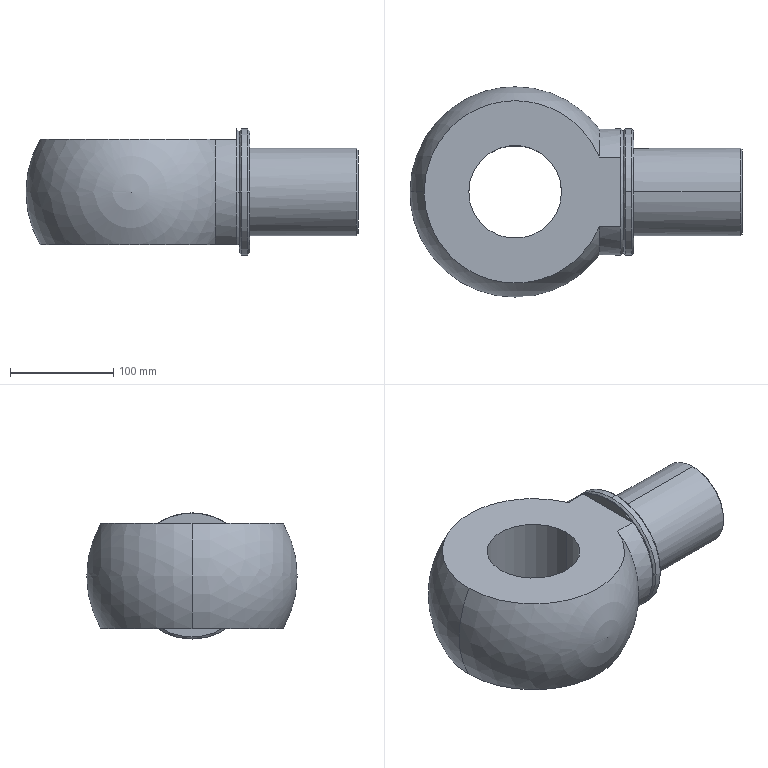Part | SolidWorks | features BaseBody 1 | 1 solid | 24 faces | box 322 x 204 x 122.4 mm | volume 3250841 mm3 | cone 9 | cylinder 7 | plane 6 | sphere 2 | commonest cylinder face diameters 122.4 x3 85 x2 90 x2
STEP:
#1=CARTESIAN_POINT('',(68.376,-42.5,0.));
#2=VERTEX_POINT('',#1);
#3=CARTESIAN_POINT('',(68.376,0.,42.5));
#4=VERTEX_POINT('',#3);
#5=CARTESIAN_POINT('',(68.376,0.,0.));
#6=DIRECTION('',(-1.,0.,0.));
#7=DIRECTION('',(0.,0.,-1.));
#8=AXIS2_PLACEMENT_3D('',#5,#6,#7);
#9=CIRCLE('',#8,42.5);
#10=EDGE_CURVE('',#2,#4,#9,.T.);
#11=ORIENTED_EDGE('',*,*,#10,.T.);
#12=CARTESIAN_POINT('',(-35.,0.,42.5));
#13=VERTEX_POINT('',#12);
#14=CARTESIAN_POINT('',(17.,0.,42.5));
#15=DIRECTION('',(-1.,0.,0.));
#16=VECTOR('',#15,1000.);
#17=LINE('',#14,#16);
#18=EDGE_CURVE('',#4,#13,#17,.T.);
#19=ORIENTED_EDGE('',*,*,#18,.T.);
#20=CARTESIAN_POINT('',(-35.,0.,-42.5));
#21=VERTEX_POINT('',#20);
#22=CARTESIAN_POINT('',(-35.,0.,0.));
#23=DIRECTION('',(-1.,0.,0.));
#24=DIRECTION('',(0.,0.,-1.));
#25=AXIS2_PLACEMENT_3D('',#22,#23,#24);
#26=CIRCLE('',#25,42.5);
#27=EDGE_CURVE('',#21,#13,#26,.T.);
#28=ORIENTED_EDGE('',*,*,#27,.F.);
#29=CARTESIAN_POINT('',(68.376,0.,-42.5));
#30=VERTEX_POINT('',#29);
#31=CARTESIAN_POINT('',(17.,0.,-42.5));
#32=DIRECTION('',(-1.,0.,0.));
#33=VECTOR('',#32,1000.);
#34=LINE('',#31,#33);
#35=EDGE_CURVE('',#30,#21,#34,.T.);
#36=ORIENTED_EDGE('',*,*,#35,.F.);
#37=CARTESIAN_POINT('',(68.376,0.,0.));
#38=DIRECTION('',(-1.,0.,0.));
#39=DIRECTION('',(0.,0.,-1.));
#40=AXIS2_PLACEMENT_3D('',#37,#38,#39);
#41=CIRCLE('',#40,42.5);
#42=EDGE_CURVE('',#30,#2,#41,.T.);
#43=ORIENTED_EDGE('',*,*,#42,.T.);
#44=EDGE_LOOP('',(#11,#19,#28,#36,#43));
#45=FACE_OUTER_BOUND('',#44,.T.);
#46=CARTESIAN_POINT('',(17.,0.,0.));
#47=DIRECTION('',(-1.,0.,0.));
#48=DIRECTION('',(0.,0.,-1.));
#49=AXIS2_PLACEMENT_3D('',#46,#47,#48);
#50=CYLINDRICAL_SURFACE('',#49,42.5);
#51=ADVANCED_FACE('',(#45),#50,.T.);
#52=CARTESIAN_POINT('',(70.,-40.876,0.));
#53=VERTEX_POINT('',#52);
#54=CARTESIAN_POINT('',(70.,40.876,0.));
#55=VERTEX_POINT('',#54);
#56=CARTESIAN_POINT('',(70.,0.,0.));
#57=DIRECTION('',(1.,0.,0.));
#58=DIRECTION('',(0.,1.,0.));
#59=AXIS2_PLACEMENT_3D('',#56,#57,#58);
#60=CIRCLE('',#59,40.876);
#61=EDGE_CURVE('',#53,#55,#60,.T.);
#62=ORIENTED_EDGE('',*,*,#61,.F.);
#63=CARTESIAN_POINT('',(69.188,-41.688,0.));
#64=DIRECTION('',(-0.7071,-0.7071,0.));
#65=VECTOR('',#64,1000.);
#66=LINE('',#63,#65);
#67=EDGE_CURVE('',#53,#2,#66,.T.);
#68=ORIENTED_EDGE('',*,*,#67,.T.);
#69=ORIENTED_EDGE('',*,*,#42,.F.);
#70=CARTESIAN_POINT('',(68.376,42.5,0.));
#71=VERTEX_POINT('',#70);
#72=CARTESIAN_POINT('',(68.376,0.,0.));
#73=DIRECTION('',(-1.,0.,0.));
#74=DIRECTION('',(0.,0.,-1.));
#75=AXIS2_PLACEMENT_3D('',#72,#73,#74);
#76=CIRCLE('',#75,42.5);
#77=EDGE_CURVE('',#71,#30,#76,.T.);
#78=ORIENTED_EDGE('',*,*,#77,.F.);
#79=CARTESIAN_POINT('',(69.188,41.688,0.));
#80=DIRECTION('',(-0.7071,0.7071,0.));
#81=VECTOR('',#80,1000.);
#82=LINE('',#79,#81);
#83=EDGE_CURVE('',#55,#71,#82,.T.);
#84=ORIENTED_EDGE('',*,*,#83,.F.);
#85=EDGE_LOOP('',(#62,#68,#69,#78,#84));
#86=FACE_OUTER_BOUND('',#85,.T.);
#87=CARTESIAN_POINT('',(69.188,0.,0.));
#88=DIRECTION('',(-1.,0.,0.));
#89=DIRECTION('',(0.,1.,0.));
#90=AXIS2_PLACEMENT_3D('',#87,#88,#89);
#91=CONICAL_SURFACE('',#90,41.688,0.7854);
#92=ADVANCED_FACE('',(#86),#91,.T.);
#93=CARTESIAN_POINT('',(-35.,-59.2,0.));
#94=VERTEX_POINT('',#93);
#95=CARTESIAN_POINT('',(-35.,59.2,0.));
#96=VERTEX_POINT('',#95);
#97=CARTESIAN_POINT('',(-35.,0.,0.));
#98=DIRECTION('',(1.,0.,0.));
#99=DIRECTION('',(0.,1.,0.));
#100=AXIS2_PLACEMENT_3D('',#97,#98,#99);
#101=CIRCLE('',#100,59.2);
#102=EDGE_CURVE('',#94,#96,#101,.T.);
#103=ORIENTED_EDGE('',*,*,#102,.F.);
#104=CARTESIAN_POINT('',(-37.,-61.2,0.));
#105=VERTEX_POINT('',#104);
#106=CARTESIAN_POINT('',(-36.,-60.2,0.));
#107=DIRECTION('',(-0.7071,-0.7071,0.));
#108=VECTOR('',#107,1000.);
#109=LINE('',#106,#108);
#110=EDGE_CURVE('',#94,#105,#109,.T.);
#111=ORIENTED_EDGE('',*,*,#110,.T.);
#112=CARTESIAN_POINT('',(-37.,0.,-61.2));
#113=VERTEX_POINT('',#112);
#114=CARTESIAN_POINT('',(-37.,0.,0.));
#115=DIRECTION('',(-1.,0.,0.));
#116=DIRECTION('',(0.,0.,-1.));
#117=AXIS2_PLACEMENT_3D('',#114,#115,#116);
#118=CIRCLE('',#117,61.2);
#119=EDGE_CURVE('',#113,#105,#118,.T.);
#120=ORIENTED_EDGE('',*,*,#119,.F.);
#121=CARTESIAN_POINT('',(-37.,61.2,0.));
#122=VERTEX_POINT('',#121);
#123=CARTESIAN_POINT('',(-37.,0.,0.));
#124=DIRECTION('',(-1.,0.,0.));
#125=DIRECTION('',(0.,0.,-1.));
#126=AXIS2_PLACEMENT_3D('',#123,#124,#125);
#127=CIRCLE('',#126,61.2);
#128=EDGE_CURVE('',#122,#113,#127,.T.);
#129=ORIENTED_EDGE('',*,*,#128,.F.);
#130=CARTESIAN_POINT('',(-36.,60.2,0.));
#131=DIRECTION('',(-0.7071,0.7071,0.));
#132=VECTOR('',#131,1000.);
#133=LINE('',#130,#132);
#134=EDGE_CURVE('',#96,#122,#133,.T.);
#135=ORIENTED_EDGE('',*,*,#134,.F.);
#136=EDGE_LOOP('',(#103,#111,#120,#129,#135));
#137=FACE_OUTER_BOUND('',#136,.T.);
#138=CARTESIAN_POINT('',(-36.,0.,0.));
#139=DIRECTION('',(-1.,0.,0.));
#140=DIRECTION('',(0.,1.,0.));
#141=AXIS2_PLACEMENT_3D('',#138,#139,#140);
#142=CONICAL_SURFACE('',#141,60.2,0.7854);
#143=ADVANCED_FACE('',(#137),#142,.T.);
#144=CARTESIAN_POINT('',(-45.,-59.2,0.));
#145=VERTEX_POINT('',#144);
#146=CARTESIAN_POINT('',(-45.,59.2,0.));
#147=VERTEX_POINT('',#146);
#148=CARTESIAN_POINT('',(-45.,0.,0.));
#149=DIRECTION('',(-1.,0.,0.));
#150=DIRECTION('',(0.,1.,0.));
#151=AXIS2_PLACEMENT_3D('',#148,#149,#150);
#152=CIRCLE('',#151,59.2);
#153=EDGE_CURVE('',#145,#147,#152,.T.);
#154=ORIENTED_EDGE('',*,*,#153,.F.);
#155=CARTESIAN_POINT('',(-43.,-61.2,0.));
#156=VERTEX_POINT('',#155);
#157=CARTESIAN_POINT('',(-44.,-60.2,0.));
#158=DIRECTION('',(0.7071,-0.7071,0.));
#159=VECTOR('',#158,1000.);
#160=LINE('',#157,#159);
#161=EDGE_CURVE('',#145,#156,#160,.T.);
#162=ORIENTED_EDGE('',*,*,#161,.T.);
#163=CARTESIAN_POINT('',(-43.,0.,61.2));
#164=VERTEX_POINT('',#163);
#165=CARTESIAN_POINT('',(-43.,0.,0.));
#166=DIRECTION('',(1.,0.,0.));
#167=DIRECTION('',(0.,0.,-1.));
#168=AXIS2_PLACEMENT_3D('',#165,#166,#167);
#169=CIRCLE('',#168,61.2);
#170=EDGE_CURVE('',#164,#156,#169,.T.);
#171=ORIENTED_EDGE('',*,*,#170,.F.);
#172=CARTESIAN_POINT('',(-43.,61.2,0.));
#173=VERTEX_POINT('',#172);
#174=CARTESIAN_POINT('',(-43.,0.,0.));
#175=DIRECTION('',(1.,0.,0.));
#176=DIRECTION('',(0.,0.,-1.));
#177=AXIS2_PLACEMENT_3D('',#174,#175,#176);
#178=CIRCLE('',#177,61.2);
#179=EDGE_CURVE('',#173,#164,#178,.T.);
#180=ORIENTED_EDGE('',*,*,#179,.F.);
#181=CARTESIAN_POINT('',(-44.,60.2,0.));
#182=DIRECTION('',(0.7071,0.7071,0.));
#183=VECTOR('',#182,1000.);
#184=LINE('',#181,#183);
#185=EDGE_CURVE('',#147,#173,#184,.T.);
#186=ORIENTED_EDGE('',*,*,#185,.F.);
#187=EDGE_LOOP('',(#154,#162,#171,#180,#186));
#188=FACE_OUTER_BOUND('',#187,.T.);
#189=CARTESIAN_POINT('',(-44.,0.,0.));
#190=DIRECTION('',(1.,0.,0.));
#191=DIRECTION('',(0.,1.,0.));
#192=AXIS2_PLACEMENT_3D('',#189,#190,#191);
#193=CONICAL_SURFACE('',#192,60.2,0.7854);
#194=ADVANCED_FACE('',(#188),#193,.T.);
#195=ORIENTED_EDGE('',*,*,#119,.T.);
#196=CARTESIAN_POINT('',(-37.,0.,61.2));
#197=VERTEX_POINT('',#196);
#198=CARTESIAN_POINT('',(-37.,0.,0.));
#199=DIRECTION('',(-1.,0.,0.));
#200=DIRECTION('',(0.,0.,-1.));
#201=AXIS2_PLACEMENT_3D('',#198,#199,#200);
#202=CIRCLE('',#201,61.2);
#203=EDGE_CURVE('',#105,#197,#202,.T.);
#204=ORIENTED_EDGE('',*,*,#203,.T.);
#205=CARTESIAN_POINT('',(-40.,0.,61.2));
#206=DIRECTION('',(-1.,0.,0.));
#207=VECTOR('',#206,1000.);
#208=LINE('',#205,#207);
#209=EDGE_CURVE('',#197,#164,#208,.T.);
#210=ORIENTED_EDGE('',*,*,#209,.T.);
#211=ORIENTED_EDGE('',*,*,#170,.T.);
#212=CARTESIAN_POINT('',(-43.,0.,-61.2));
#213=VERTEX_POINT('',#212);
#214=CARTESIAN_POINT('',(-43.,0.,0.));
#215=DIRECTION('',(1.,0.,0.));
#216=DIRECTION('',(0.,0.,-1.));
#217=AXIS2_PLACEMENT_3D('',#214,#215,#216);
#218=CIRCLE('',#217,61.2);
#219=EDGE_CURVE('',#156,#213,#218,.T.);
#220=ORIENTED_EDGE('',*,*,#219,.T.);
#221=CARTESIAN_POINT('',(-40.,0.,-61.2));
#222=DIRECTION('',(-1.,0.,0.));
#223=VECTOR('',#222,1000.);
#224=LINE('',#221,#223);
#225=EDGE_CURVE('',#113,#213,#224,.T.);
#226=ORIENTED_EDGE('',*,*,#225,.F.);
#227=EDGE_LOOP('',(#195,#204,#210,#211,#220,#226));
#228=FACE_OUTER_BOUND('',#227,.T.);
#229=CARTESIAN_POINT('',(-40.,0.,0.));
#230=DIRECTION('',(-1.,0.,0.));
#231=DIRECTION('',(0.,0.,-1.));
#232=AXIS2_PLACEMENT_3D('',#229,#230,#231);
#233=CYLINDRICAL_SURFACE('',#232,61.2);
#234=ADVANCED_FACE('',(#228),#233,.T.);
#235=CARTESIAN_POINT('',(-105.,0.,-51.));
#236=VERTEX_POINT('',#235);
#237=CARTESIAN_POINT('',(-195.,0.,-51.));
#238=VERTEX_POINT('',#237);
#239=CARTESIAN_POINT('',(-150.,0.,-51.));
#240=DIRECTION('',(0.,0.,1.));
#241=DIRECTION('',(-1.,0.,0.));
#242=AXIS2_PLACEMENT_3D('',#239,#240,#241);
#243=CIRCLE('',#242,45.);
#244=EDGE_CURVE('',#236,#238,#243,.T.);
#245=ORIENTED_EDGE('',*,*,#244,.F.);
#246=CARTESIAN_POINT('',(-105.,0.,51.));
#247=VERTEX_POINT('',#246);
#248=CARTESIAN_POINT('',(-105.,0.,0.));
#249=DIRECTION('',(0.,0.,1.));
#250=VECTOR('',#249,1000.);
#251=LINE('',#248,#250);
#252=EDGE_CURVE('',#236,#247,#251,.T.);
#253=ORIENTED_EDGE('',*,*,#252,.T.);
#254=CARTESIAN_POINT('',(-195.,0.,51.));
#255=VERTEX_POINT('',#254);
#256=CARTESIAN_POINT('',(-150.,0.,51.));
#257=DIRECTION('',(0.,0.,-1.));
#258=DIRECTION('',(-1.,0.,0.));
#259=AXIS2_PLACEMENT_3D('',#256,#257,#258);
#260=CIRCLE('',#259,45.);
#261=EDGE_CURVE('',#255,#247,#260,.T.);
#262=ORIENTED_EDGE('',*,*,#261,.F.);
#263=CARTESIAN_POINT('',(-195.,0.,0.));
#264=DIRECTION('',(0.,0.,1.));
#265=VECTOR('',#264,1000.);
#266=LINE('',#263,#265);
#267=EDGE_CURVE('',#238,#255,#266,.T.);
#268=ORIENTED_EDGE('',*,*,#267,.F.);
#269=EDGE_LOOP('',(#245,#253,#262,#268));
#270=FACE_OUTER_BOUND('',#269,.T.);
#271=CARTESIAN_POINT('',(-150.,0.,0.));
#272=DIRECTION('',(0.,0.,1.));
#273=DIRECTION('',(-1.,0.,0.));
#274=AXIS2_PLACEMENT_3D('',#271,#272,#273);
#275=CYLINDRICAL_SURFACE('',#274,45.);
#276=ADVANCED_FACE('',(#270),#275,.F.);
#277=CARTESIAN_POINT('',(-45.,-58.752,0.));
#278=VERTEX_POINT('',#277);
#279=CARTESIAN_POINT('',(-45.,-29.168,-51.));
#280=VERTEX_POINT('',#279);
#281=CARTESIAN_POINT('',(-45.,0.,0.));
#282=DIRECTION('',(1.,0.,0.));
#283=DIRECTION('',(0.,1.,0.));
#284=AXIS2_PLACEMENT_3D('',#281,#282,#283);
#285=CIRCLE('',#284,58.752);
#286=EDGE_CURVE('',#278,#280,#285,.T.);
#287=ORIENTED_EDGE('',*,*,#286,.F.);
#288=CARTESIAN_POINT('',(-47.448,-61.2,0.));
#289=VERTEX_POINT('',#288);
#290=CARTESIAN_POINT('',(-46.224,-59.976,0.));
#291=DIRECTION('',(-0.7071,-0.7071,0.));
#292=VECTOR('',#291,1000.);
#293=LINE('',#290,#292);
#294=EDGE_CURVE('',#278,#289,#293,.T.);
#295=ORIENTED_EDGE('',*,*,#294,.T.);
#296=CARTESIAN_POINT('',(-47.448,-33.83,-51.));
#297=VERTEX_POINT('',#296);
#298=CARTESIAN_POINT('',(-47.448,0.,0.));
#299=DIRECTION('',(-1.,0.,0.));
#300=DIRECTION('',(0.,0.,-1.));
#301=AXIS2_PLACEMENT_3D('',#298,#299,#300);
#302=CIRCLE('',#301,61.2);
#303=EDGE_CURVE('',#297,#289,#302,.T.);
#304=ORIENTED_EDGE('',*,*,#303,.F.);
#305=CARTESIAN_POINT('',(-47.448,-33.83,-51.));
#306=CARTESIAN_POINT('',(-46.133,-31.451,-51.));
#307=CARTESIAN_POINT('',(-45.,-29.168,-51.));
#308=(BOUNDED_CURVE()B_SPLINE_CURVE(2,(#305,#306,#307),.UNSPECIFIED.,.F.,.F.)B_SPLINE_CURVE_WITH_KNOTS((3,3),(0.,5.265),.UNSPECIFIED.)CURVE()GEOMETRIC_REPRESENTATION_ITEM()RATIONAL_B_SPLINE_CURVE((1.,1.001,1.))REPRESENTATION_ITEM(''));
#309=EDGE_CURVE('',#297,#280,#308,.T.);
#310=ORIENTED_EDGE('',*,*,#309,.T.);
#311=EDGE_LOOP('',(#287,#295,#304,#310));
#312=FACE_OUTER_BOUND('',#311,.T.);
#313=CARTESIAN_POINT('',(-46.224,0.,0.));
#314=DIRECTION('',(-1.,0.,0.));
#315=DIRECTION('',(0.,1.,0.));
#316=AXIS2_PLACEMENT_3D('',#313,#314,#315);
#317=CONICAL_SURFACE('',#316,59.976,0.7854);
#318=ADVANCED_FACE('',(#312),#317,.T.);
#319=ORIENTED_EDGE('',*,*,#294,.F.);
#320=CARTESIAN_POINT('',(-45.,58.752,0.));
#321=VERTEX_POINT('',#320);
#322=CARTESIAN_POINT('',(-45.,0.,0.));
#323=DIRECTION('',(1.,0.,0.));
#324=DIRECTION('',(0.,1.,0.));
#325=AXIS2_PLACEMENT_3D('',#322,#323,#324);
#326=CIRCLE('',#325,58.752);
#327=EDGE_CURVE('',#321,#278,#326,.T.);
#328=ORIENTED_EDGE('',*,*,#327,.F.);
#329=CARTESIAN_POINT('',(-47.448,61.2,0.));
#330=VERTEX_POINT('',#329);
#331=CARTESIAN_POINT('',(-46.224,59.976,0.));
#332=DIRECTION('',(-0.7071,0.7071,0.));
#333=VECTOR('',#332,1000.);
#334=LINE('',#331,#333);
#335=EDGE_CURVE('',#321,#330,#334,.T.);
#336=ORIENTED_EDGE('',*,*,#335,.T.);
#337=CARTESIAN_POINT('',(-47.448,0.,0.));
#338=DIRECTION('',(-1.,0.,0.));
#339=DIRECTION('',(0.,0.,-1.));
#340=AXIS2_PLACEMENT_3D('',#337,#338,#339);
#341=CIRCLE('',#340,61.2);
#342=EDGE_CURVE('',#289,#330,#341,.T.);
#343=ORIENTED_EDGE('',*,*,#342,.F.);
#344=EDGE_LOOP('',(#319,#328,#336,#343));
#345=FACE_OUTER_BOUND('',#344,.T.);
#346=CARTESIAN_POINT('',(-46.224,0.,0.));
#347=DIRECTION('',(-1.,0.,0.));
#348=DIRECTION('',(0.,1.,0.));
#349=AXIS2_PLACEMENT_3D('',#346,#347,#348);
#350=CONICAL_SURFACE('',#349,59.976,0.7854);
#351=ADVANCED_FACE('',(#345),#350,.T.);
#352=CARTESIAN_POINT('',(-68.4,-33.83,51.));
#353=VERTEX_POINT('',#352);
#354=CARTESIAN_POINT('',(-238.335,0.,51.));
#355=VERTEX_POINT('',#354);
#356=CARTESIAN_POINT('',(-150.,0.,51.));
#357=DIRECTION('',(0.,0.,-1.));
#358=DIRECTION('',(0.,1.,0.));
#359=AXIS2_PLACEMENT_3D('',#356,#357,#358);
#360=CIRCLE('',#359,88.335);
#361=EDGE_CURVE('',#353,#355,#360,.T.);
#362=ORIENTED_EDGE('',*,*,#361,.T.);
#363=CARTESIAN_POINT('',(-238.335,0.,-51.));
#364=VERTEX_POINT('',#363);
#365=CARTESIAN_POINT('',(-150.,0.,0.));
#366=DIRECTION('',(0.,-1.,0.));
#367=DIRECTION('',(0.,0.,-1.));
#368=AXIS2_PLACEMENT_3D('',#365,#366,#367);
#369=CIRCLE('',#368,102.);
#370=EDGE_CURVE('',#355,#364,#369,.T.);
#371=ORIENTED_EDGE('',*,*,#370,.T.);
#372=CARTESIAN_POINT('',(-68.4,-33.83,-51.));
#373=VERTEX_POINT('',#372);
#374=CARTESIAN_POINT('',(-150.,0.,-51.));
#375=DIRECTION('',(0.,0.,1.));
#376=DIRECTION('',(0.,-1.,0.));
#377=AXIS2_PLACEMENT_3D('',#374,#375,#376);
#378=CIRCLE('',#377,88.335);
#379=EDGE_CURVE('',#364,#373,#378,.T.);
#380=ORIENTED_EDGE('',*,*,#379,.T.);
#381=CARTESIAN_POINT('',(-68.4,0.,0.));
#382=DIRECTION('',(-1.,0.,0.));
#383=DIRECTION('',(0.,0.,-1.));
#384=AXIS2_PLACEMENT_3D('',#381,#382,#383);
#385=CIRCLE('',#384,61.2);
#386=EDGE_CURVE('',#373,#353,#385,.T.);
#387=ORIENTED_EDGE('',*,*,#386,.T.);
#388=EDGE_LOOP('',(#362,#371,#380,#387));
#389=FACE_OUTER_BOUND('',#388,.T.);
#390=CARTESIAN_POINT('',(-150.,0.,0.));
#391=DIRECTION('',(0.,1.,0.));
#392=DIRECTION('',(-1.,0.,0.));
#393=AXIS2_PLACEMENT_3D('',#390,#391,#392);
#394=SPHERICAL_SURFACE('',#393,102.);
#395=ADVANCED_FACE('',(#389),#394,.T.);
#396=ORIENTED_EDGE('',*,*,#370,.F.);
#397=CARTESIAN_POINT('',(-68.4,33.83,51.));
#398=VERTEX_POINT('',#397);
#399=CARTESIAN_POINT('',(-150.,0.,51.));
#400=DIRECTION('',(0.,0.,-1.));
#401=DIRECTION('',(0.,1.,0.));
#402=AXIS2_PLACEMENT_3D('',#399,#400,#401);
#403=CIRCLE('',#402,88.335);
#404=EDGE_CURVE('',#355,#398,#403,.T.);
#405=ORIENTED_EDGE('',*,*,#404,.T.);
#406=CARTESIAN_POINT('',(-68.4,33.83,-51.));
#407=VERTEX_POINT('',#406);
#408=CARTESIAN_POINT('',(-68.4,0.,0.));
#409=DIRECTION('',(-1.,0.,0.));
#410=DIRECTION('',(0.,0.,-1.));
#411=AXIS2_PLACEMENT_3D('',#408,#409,#410);
#412=CIRCLE('',#411,61.2);
#413=EDGE_CURVE('',#398,#407,#412,.T.);
#414=ORIENTED_EDGE('',*,*,#413,.T.);
#415=CARTESIAN_POINT('',(-150.,0.,-51.));
#416=DIRECTION('',(0.,0.,1.));
#417=DIRECTION('',(0.,-1.,0.));
#418=AXIS2_PLACEMENT_3D('',#415,#416,#417);
#419=CIRCLE('',#418,88.335);
#420=EDGE_CURVE('',#407,#364,#419,.T.);
#421=ORIENTED_EDGE('',*,*,#420,.T.);
#422=EDGE_LOOP('',(#396,#405,#414,#421));
#423=FACE_OUTER_BOUND('',#422,.T.);
#424=CARTESIAN_POINT('',(-150.,0.,0.));
#425=DIRECTION('',(0.,1.,0.));
#426=DIRECTION('',(-1.,0.,0.));
#427=AXIS2_PLACEMENT_3D('',#424,#425,#426);
#428=SPHERICAL_SURFACE('',#427,102.);
#429=ADVANCED_FACE('',(#423),#428,.T.);
#430=ORIENTED_EDGE('',*,*,#335,.F.);
#431=CARTESIAN_POINT('',(-45.,29.168,-51.));
#432=VERTEX_POINT('',#431);
#433=CARTESIAN_POINT('',(-45.,0.,0.));
#434=DIRECTION('',(1.,0.,0.));
#435=DIRECTION('',(0.,1.,0.));
#436=AXIS2_PLACEMENT_3D('',#433,#434,#435);
#437=CIRCLE('',#436,58.752);
#438=EDGE_CURVE('',#432,#321,#437,.T.);
#439=ORIENTED_EDGE('',*,*,#438,.F.);
#440=CARTESIAN_POINT('',(-47.448,33.83,-51.));
#441=VERTEX_POINT('',#440);
#442=CARTESIAN_POINT('',(-45.,29.168,-51.));
#443=CARTESIAN_POINT('',(-46.133,31.451,-51.));
#444=CARTESIAN_POINT('',(-47.448,33.83,-51.));
#445=(BOUNDED_CURVE()B_SPLINE_CURVE(2,(#442,#443,#444),.UNSPECIFIED.,.F.,.F.)B_SPLINE_CURVE_WITH_KNOTS((3,3),(0.,5.265),.UNSPECIFIED.)CURVE()GEOMETRIC_REPRESENTATION_ITEM()RATIONAL_B_SPLINE_CURVE((1.,1.001,1.))REPRESENTATION_ITEM(''));
#446=EDGE_CURVE('',#432,#441,#445,.T.);
#447=ORIENTED_EDGE('',*,*,#446,.T.);
#448=CARTESIAN_POINT('',(-47.448,0.,0.));
#449=DIRECTION('',(-1.,0.,0.));
#450=DIRECTION('',(0.,0.,-1.));
#451=AXIS2_PLACEMENT_3D('',#448,#449,#450);
#452=CIRCLE('',#451,61.2);
#453=EDGE_CURVE('',#330,#441,#452,.T.);
#454=ORIENTED_EDGE('',*,*,#453,.F.);
#455=EDGE_LOOP('',(#430,#439,#447,#454));
#456=FACE_OUTER_BOUND('',#455,.T.);
#457=CARTESIAN_POINT('',(-46.224,0.,0.));
#458=DIRECTION('',(-1.,0.,0.));
#459=DIRECTION('',(0.,1.,0.));
#460=AXIS2_PLACEMENT_3D('',#457,#458,#459);
#461=CONICAL_SURFACE('',#460,59.976,0.7854);
#462=ADVANCED_FACE('',(#456),#461,.T.);
#463=ORIENTED_EDGE('',*,*,#309,.F.);
#464=CARTESIAN_POINT('',(-57.924,-33.83,-51.));
#465=DIRECTION('',(1.,0.,0.));
#466=VECTOR('',#465,1000.);
#467=LINE('',#464,#466);
#468=EDGE_CURVE('',#373,#297,#467,.T.);
#469=ORIENTED_EDGE('',*,*,#468,.F.);
#470=ORIENTED_EDGE('',*,*,#379,.F.);
#471=ORIENTED_EDGE('',*,*,#420,.F.);
#472=CARTESIAN_POINT('',(-57.924,33.83,-51.));
#473=DIRECTION('',(-1.,0.,0.));
#474=VECTOR('',#473,1000.);
#475=LINE('',#472,#474);
#476=EDGE_CURVE('',#441,#407,#475,.T.);
#477=ORIENTED_EDGE('',*,*,#476,.F.);
#478=ORIENTED_EDGE('',*,*,#446,.F.);
#479=CARTESIAN_POINT('',(-45.,0.,-51.));
#480=DIRECTION('',(0.,1.,0.));
#481=VECTOR('',#480,1000.);
#482=LINE('',#479,#481);
#483=EDGE_CURVE('',#280,#432,#482,.T.);
#484=ORIENTED_EDGE('',*,*,#483,.F.);
#485=EDGE_LOOP('',(#463,#469,#470,#471,#477,#478,#484));
#486=FACE_OUTER_BOUND('',#485,.T.);
#487=CARTESIAN_POINT('',(-150.,0.,-51.));
#488=DIRECTION('',(0.,0.,1.));
#489=DIRECTION('',(-1.,0.,0.));
#490=AXIS2_PLACEMENT_3D('',#487,#488,#489);
#491=CIRCLE('',#490,45.);
#492=EDGE_CURVE('',#238,#236,#491,.T.);
#493=ORIENTED_EDGE('',*,*,#492,.T.);
#494=ORIENTED_EDGE('',*,*,#244,.T.);
#495=EDGE_LOOP('',(#493,#494));
#496=FACE_BOUND('',#495,.T.);
#497=CARTESIAN_POINT('',(-148.5,0.,-51.));
#498=DIRECTION('',(0.,0.,-1.));
#499=DIRECTION('',(-1.,0.,0.));
#500=AXIS2_PLACEMENT_3D('',#497,#498,#499);
#501=PLANE('',#500);
#502=ADVANCED_FACE('',(#486,#496),#501,.T.);
#503=CARTESIAN_POINT('',(-48.,33.83,51.));
#504=VERTEX_POINT('',#503);
#505=CARTESIAN_POINT('',(-58.2,33.83,51.));
#506=DIRECTION('',(1.,0.,0.));
#507=VECTOR('',#506,1000.);
#508=LINE('',#505,#507);
#509=EDGE_CURVE('',#398,#504,#508,.T.);
#510=ORIENTED_EDGE('',*,*,#509,.T.);
#511=CARTESIAN_POINT('',(-48.,-33.83,51.));
#512=VERTEX_POINT('',#511);
#513=CARTESIAN_POINT('',(-48.,0.,0.));
#514=DIRECTION('',(1.,0.,0.));
#515=DIRECTION('',(0.,0.,-1.));
#516=AXIS2_PLACEMENT_3D('',#513,#514,#515);
#517=CIRCLE('',#516,61.2);
#518=EDGE_CURVE('',#504,#512,#517,.T.);
#519=ORIENTED_EDGE('',*,*,#518,.T.);
#520=CARTESIAN_POINT('',(-58.2,-33.83,51.));
#521=DIRECTION('',(-1.,0.,0.));
#522=VECTOR('',#521,1000.);
#523=LINE('',#520,#522);
#524=EDGE_CURVE('',#512,#353,#523,.T.);
#525=ORIENTED_EDGE('',*,*,#524,.T.);
#526=ORIENTED_EDGE('',*,*,#386,.F.);
#527=ORIENTED_EDGE('',*,*,#468,.T.);
#528=ORIENTED_EDGE('',*,*,#303,.T.);
#529=ORIENTED_EDGE('',*,*,#342,.T.);
#530=ORIENTED_EDGE('',*,*,#453,.T.);
#531=ORIENTED_EDGE('',*,*,#476,.T.);
#532=ORIENTED_EDGE('',*,*,#413,.F.);
#533=EDGE_LOOP('',(#510,#519,#525,#526,#527,#528,#529,#530,#531,#532));
#534=FACE_OUTER_BOUND('',#533,.T.);
#535=CARTESIAN_POINT('',(-97.5,0.,0.));
#536=DIRECTION('',(-1.,0.,0.));
#537=DIRECTION('',(0.,0.,-1.));
#538=AXIS2_PLACEMENT_3D('',#535,#536,#537);
#539=CYLINDRICAL_SURFACE('',#538,61.2);
#540=ADVANCED_FACE('',(#534),#539,.T.);
#541=ORIENTED_EDGE('',*,*,#509,.F.);
#542=ORIENTED_EDGE('',*,*,#404,.F.);
#543=ORIENTED_EDGE('',*,*,#361,.F.);
#544=ORIENTED_EDGE('',*,*,#524,.F.);
#545=CARTESIAN_POINT('',(-48.,0.,51.));
#546=DIRECTION('',(0.,-1.,0.));
#547=VECTOR('',#546,1000.);
#548=LINE('',#545,#547);
#549=EDGE_CURVE('',#504,#512,#548,.T.);
#550=ORIENTED_EDGE('',*,*,#549,.F.);
#551=EDGE_LOOP('',(#541,#542,#543,#544,#550));
#552=FACE_OUTER_BOUND('',#551,.T.);
#553=ORIENTED_EDGE('',*,*,#261,.T.);
#554=CARTESIAN_POINT('',(-150.,0.,51.));
#555=DIRECTION('',(0.,0.,-1.));
#556=DIRECTION('',(-1.,0.,0.));
#557=AXIS2_PLACEMENT_3D('',#554,#555,#556);
#558=CIRCLE('',#557,45.);
#559=EDGE_CURVE('',#247,#255,#558,.T.);
#560=ORIENTED_EDGE('',*,*,#559,.T.);
#561=EDGE_LOOP('',(#553,#560));
#562=FACE_BOUND('',#561,.T.);
#563=CARTESIAN_POINT('',(-151.5,0.,51.));
#564=DIRECTION('',(0.,0.,1.));
#565=DIRECTION('',(1.,0.,0.));
#566=AXIS2_PLACEMENT_3D('',#563,#564,#565);
#567=PLANE('',#566);
#568=ADVANCED_FACE('',(#552,#562),#567,.T.);
#569=ORIENTED_EDGE('',*,*,#518,.F.);
#570=ORIENTED_EDGE('',*,*,#549,.T.);
#571=EDGE_LOOP('',(#569,#570));
#572=FACE_OUTER_BOUND('',#571,.T.);
#573=CARTESIAN_POINT('',(-48.,0.,102.));
#574=DIRECTION('',(-1.,0.,0.));
#575=DIRECTION('',(0.,0.,1.));
#576=AXIS2_PLACEMENT_3D('',#573,#574,#575);
#577=PLANE('',#576);
#578=ADVANCED_FACE('',(#572),#577,.T.);
#579=ORIENTED_EDGE('',*,*,#252,.F.);
#580=ORIENTED_EDGE('',*,*,#492,.F.);
#581=ORIENTED_EDGE('',*,*,#267,.T.);
#582=ORIENTED_EDGE('',*,*,#559,.F.);
#583=EDGE_LOOP('',(#579,#580,#581,#582));
#584=FACE_OUTER_BOUND('',#583,.T.);
#585=CARTESIAN_POINT('',(-150.,0.,0.));
#586=DIRECTION('',(0.,0.,1.));
#587=DIRECTION('',(-1.,0.,0.));
#588=AXIS2_PLACEMENT_3D('',#585,#586,#587);
#589=CYLINDRICAL_SURFACE('',#588,45.);
#590=ADVANCED_FACE('',(#584),#589,.F.);
#591=CARTESIAN_POINT('',(-35.,0.,0.));
#592=DIRECTION('',(1.,0.,0.));
#593=DIRECTION('',(0.,1.,0.));
#594=AXIS2_PLACEMENT_3D('',#591,#592,#593);
#595=CIRCLE('',#594,59.2);
#596=EDGE_CURVE('',#96,#94,#595,.T.);
#597=ORIENTED_EDGE('',*,*,#596,.T.);
#598=ORIENTED_EDGE('',*,*,#102,.T.);
#599=EDGE_LOOP('',(#597,#598));
#600=FACE_OUTER_BOUND('',#599,.T.);
#601=ORIENTED_EDGE('',*,*,#27,.T.);
#602=CARTESIAN_POINT('',(-35.,0.,0.));
#603=DIRECTION('',(-1.,0.,0.));
#604=DIRECTION('',(0.,0.,-1.));
#605=AXIS2_PLACEMENT_3D('',#602,#603,#604);
#606=CIRCLE('',#605,42.5);
#607=EDGE_CURVE('',#13,#21,#606,.T.);
#608=ORIENTED_EDGE('',*,*,#607,.T.);
#609=EDGE_LOOP('',(#601,#608));
#610=FACE_BOUND('',#609,.T.);
#611=CARTESIAN_POINT('',(-35.,0.,0.));
#612=DIRECTION('',(1.,0.,0.));
#613=DIRECTION('',(0.,0.,-1.));
#614=AXIS2_PLACEMENT_3D('',#611,#612,#613);
#615=PLANE('',#614);
#616=ADVANCED_FACE('',(#600,#610),#615,.T.);
#617=ORIENTED_EDGE('',*,*,#209,.F.);
#618=CARTESIAN_POINT('',(-37.,0.,0.));
#619=DIRECTION('',(-1.,0.,0.));
#620=DIRECTION('',(0.,0.,-1.));
#621=AXIS2_PLACEMENT_3D('',#618,#619,#620);
#622=CIRCLE('',#621,61.2);
#623=EDGE_CURVE('',#197,#122,#622,.T.);
#624=ORIENTED_EDGE('',*,*,#623,.T.);
#625=ORIENTED_EDGE('',*,*,#128,.T.);
#626=ORIENTED_EDGE('',*,*,#225,.T.);
#627=CARTESIAN_POINT('',(-43.,0.,0.));
#628=DIRECTION('',(1.,0.,0.));
#629=DIRECTION('',(0.,0.,-1.));
#630=AXIS2_PLACEMENT_3D('',#627,#628,#629);
#631=CIRCLE('',#630,61.2);
#632=EDGE_CURVE('',#213,#173,#631,.T.);
#633=ORIENTED_EDGE('',*,*,#632,.T.);
#634=ORIENTED_EDGE('',*,*,#179,.T.);
#635=EDGE_LOOP('',(#617,#624,#625,#626,#633,#634));
#636=FACE_OUTER_BOUND('',#635,.T.);
#637=CARTESIAN_POINT('',(-40.,0.,0.));
#638=DIRECTION('',(-1.,0.,0.));
#639=DIRECTION('',(0.,0.,-1.));
#640=AXIS2_PLACEMENT_3D('',#637,#638,#639);
#641=CYLINDRICAL_SURFACE('',#640,61.2);
#642=ADVANCED_FACE('',(#636),#641,.T.);
#643=ORIENTED_EDGE('',*,*,#161,.F.);
#644=CARTESIAN_POINT('',(-45.,0.,0.));
#645=DIRECTION('',(-1.,0.,0.));
#646=DIRECTION('',(0.,1.,0.));
#647=AXIS2_PLACEMENT_3D('',#644,#645,#646);
#648=CIRCLE('',#647,59.2);
#649=EDGE_CURVE('',#147,#145,#648,.T.);
#650=ORIENTED_EDGE('',*,*,#649,.F.);
#651=ORIENTED_EDGE('',*,*,#185,.T.);
#652=ORIENTED_EDGE('',*,*,#632,.F.);
#653=ORIENTED_EDGE('',*,*,#219,.F.);
#654=EDGE_LOOP('',(#643,#650,#651,#652,#653));
#655=FACE_OUTER_BOUND('',#654,.T.);
#656=CARTESIAN_POINT('',(-44.,0.,0.));
#657=DIRECTION('',(1.,0.,0.));
#658=DIRECTION('',(0.,1.,0.));
#659=AXIS2_PLACEMENT_3D('',#656,#657,#658);
#660=CONICAL_SURFACE('',#659,60.2,0.7854);
#661=ADVANCED_FACE('',(#655),#660,.T.);
#662=ORIENTED_EDGE('',*,*,#110,.F.);
#663=ORIENTED_EDGE('',*,*,#596,.F.);
#664=ORIENTED_EDGE('',*,*,#134,.T.);
#665=ORIENTED_EDGE('',*,*,#623,.F.);
#666=ORIENTED_EDGE('',*,*,#203,.F.);
#667=EDGE_LOOP('',(#662,#663,#664,#665,#666));
#668=FACE_OUTER_BOUND('',#667,.T.);
#669=CARTESIAN_POINT('',(-36.,0.,0.));
#670=DIRECTION('',(-1.,0.,0.));
#671=DIRECTION('',(0.,1.,0.));
#672=AXIS2_PLACEMENT_3D('',#669,#670,#671);
#673=CONICAL_SURFACE('',#672,60.2,0.7854);
#674=ADVANCED_FACE('',(#668),#673,.T.);
#675=ORIENTED_EDGE('',*,*,#483,.T.);
#676=ORIENTED_EDGE('',*,*,#438,.T.);
#677=ORIENTED_EDGE('',*,*,#327,.T.);
#678=ORIENTED_EDGE('',*,*,#286,.T.);
#679=EDGE_LOOP('',(#675,#676,#677,#678));
#680=FACE_BOUND('',#679,.T.);
#681=ORIENTED_EDGE('',*,*,#649,.T.);
#682=ORIENTED_EDGE('',*,*,#153,.T.);
#683=EDGE_LOOP('',(#681,#682));
#684=FACE_OUTER_BOUND('',#683,.T.);
#685=CARTESIAN_POINT('',(-45.,0.,0.));
#686=DIRECTION('',(-1.,0.,0.));
#687=DIRECTION('',(0.,0.,1.));
#688=AXIS2_PLACEMENT_3D('',#685,#686,#687);
#689=PLANE('',#688);
#690=ADVANCED_FACE('',(#680,#684),#689,.T.);
#691=CARTESIAN_POINT('',(70.,0.,0.));
#692=DIRECTION('',(1.,0.,0.));
#693=DIRECTION('',(0.,1.,0.));
#694=AXIS2_PLACEMENT_3D('',#691,#692,#693);
#695=CIRCLE('',#694,40.876);
#696=EDGE_CURVE('',#55,#53,#695,.T.);
#697=ORIENTED_EDGE('',*,*,#696,.T.);
#698=ORIENTED_EDGE('',*,*,#61,.T.);
#699=EDGE_LOOP('',(#697,#698));
#700=FACE_OUTER_BOUND('',#699,.T.);
#701=CARTESIAN_POINT('',(70.,0.,0.));
#702=DIRECTION('',(1.,0.,0.));
#703=DIRECTION('',(0.,0.,-1.));
#704=AXIS2_PLACEMENT_3D('',#701,#702,#703);
#705=PLANE('',#704);
#706=ADVANCED_FACE('',(#700),#705,.T.);
#707=ORIENTED_EDGE('',*,*,#67,.F.);
#708=ORIENTED_EDGE('',*,*,#696,.F.);
#709=ORIENTED_EDGE('',*,*,#83,.T.);
#710=CARTESIAN_POINT('',(68.376,0.,0.));
#711=DIRECTION('',(-1.,0.,0.));
#712=DIRECTION('',(0.,0.,-1.));
#713=AXIS2_PLACEMENT_3D('',#710,#711,#712);
#714=CIRCLE('',#713,42.5);
#715=EDGE_CURVE('',#4,#71,#714,.T.);
#716=ORIENTED_EDGE('',*,*,#715,.F.);
#717=ORIENTED_EDGE('',*,*,#10,.F.);
#718=EDGE_LOOP('',(#707,#708,#709,#716,#717));
#719=FACE_OUTER_BOUND('',#718,.T.);
#720=CARTESIAN_POINT('',(69.188,0.,0.));
#721=DIRECTION('',(-1.,0.,0.));
#722=DIRECTION('',(0.,1.,0.));
#723=AXIS2_PLACEMENT_3D('',#720,#721,#722);
#724=CONICAL_SURFACE('',#723,41.688,0.7854);
#725=ADVANCED_FACE('',(#719),#724,.T.);
#726=ORIENTED_EDGE('',*,*,#18,.F.);
#727=ORIENTED_EDGE('',*,*,#715,.T.);
#728=ORIENTED_EDGE('',*,*,#77,.T.);
#729=ORIENTED_EDGE('',*,*,#35,.T.);
#730=ORIENTED_EDGE('',*,*,#607,.F.);
#731=EDGE_LOOP('',(#726,#727,#728,#729,#730));
#732=FACE_OUTER_BOUND('',#731,.T.);
#733=CARTESIAN_POINT('',(17.,0.,0.));
#734=DIRECTION('',(-1.,0.,0.));
#735=DIRECTION('',(0.,0.,-1.));
#736=AXIS2_PLACEMENT_3D('',#733,#734,#735);
#737=CYLINDRICAL_SURFACE('',#736,42.5);
#738=ADVANCED_FACE('',(#732),#737,.T.);
#739=CLOSED_SHELL('',(#51,#92,#143,#194,#234,#276,#318,#351,#395,#429,#462,#502,#540,#568,#578,#590,#616,#642,#661,#674,#690,#706,#725,#738));
#740=MANIFOLD_SOLID_BREP('',#739);
#741=CARTESIAN_POINT('',(0.,0.,0.));
#742=DIRECTION('',(0.,0.,1.));
#743=DIRECTION('',(1.,0.,0.));
#744=AXIS2_PLACEMENT_3D('',#741,#742,#743);
#745=(LENGTH_UNIT()NAMED_UNIT(*)SI_UNIT(.MILLI.,.METRE.));
#746=UNCERTAINTY_MEASURE_WITH_UNIT(LENGTH_MEASURE(0.00001),#745,'','');
#747=(NAMED_UNIT(*)PLANE_ANGLE_UNIT()SI_UNIT($,.RADIAN.));
#748=(NAMED_UNIT(*)SI_UNIT($,.STERADIAN.)SOLID_ANGLE_UNIT());
#749=(GEOMETRIC_REPRESENTATION_CONTEXT(3)GLOBAL_UNCERTAINTY_ASSIGNED_CONTEXT((#746))GLOBAL_UNIT_ASSIGNED_CONTEXT((#745,#747,#748))REPRESENTATION_CONTEXT('',''));
#750=ADVANCED_BREP_SHAPE_REPRESENTATION('',(#740,#744),#749);